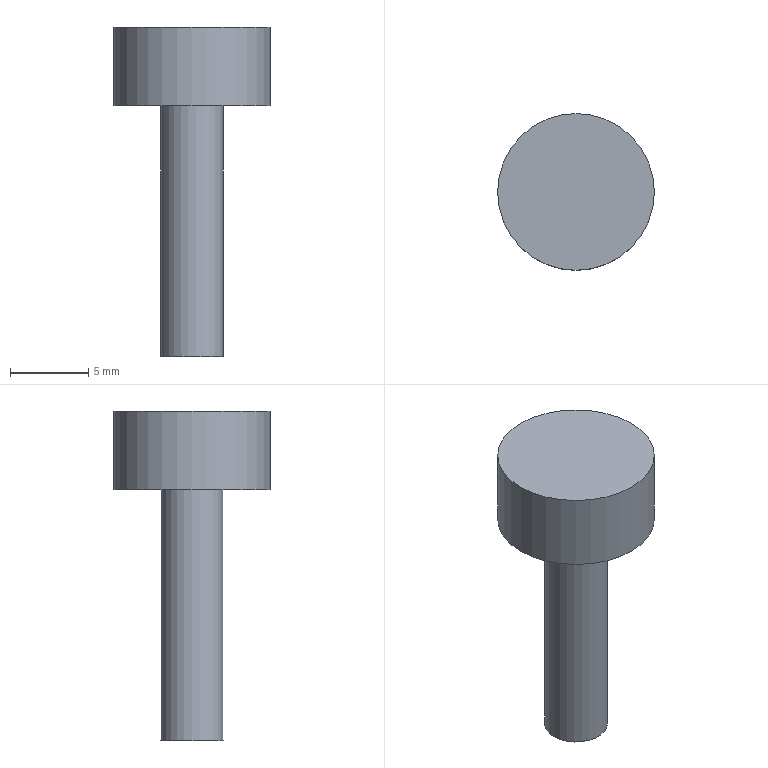Part | NX | features CYLINDER 2, DATUM_CSYS 1 | 1 solid | 5 faces | box 10 x 10 x 21 mm | volume 593.761 mm3 | plane 3 | cylinder 2 | commonest cylinder face diameters 4 x1 10 x1
STEP:
#1=CARTESIAN_POINT('',(2.,0.,0.));
#2=VERTEX_POINT('',#1);
#3=CARTESIAN_POINT('',(0.,0.,0.));
#4=DIRECTION('',(0.,0.,1.));
#5=DIRECTION('',(1.,0.,0.));
#6=AXIS2_PLACEMENT_3D('',#3,#4,#5);
#7=CIRCLE('',#6,2.);
#8=EDGE_CURVE('',#2,#2,#7,.T.);
#9=ORIENTED_EDGE('',*,*,#8,.F.);
#10=EDGE_LOOP('',(#9));
#11=FACE_BOUND('',#10,.T.);
#12=CARTESIAN_POINT('',(0.,0.,0.));
#13=DIRECTION('',(0.,0.,-1.));
#14=DIRECTION('',(-1.,0.,0.));
#15=AXIS2_PLACEMENT_3D('',#12,#13,#14);
#16=PLANE('',#15);
#17=ADVANCED_FACE('',(#11),#16,.T.);
#18=CARTESIAN_POINT('',(2.,0.,16.));
#19=VERTEX_POINT('',#18);
#20=CARTESIAN_POINT('',(0.,0.,16.));
#21=DIRECTION('',(0.,0.,-1.));
#22=DIRECTION('',(1.,0.,0.));
#23=AXIS2_PLACEMENT_3D('',#20,#21,#22);
#24=CIRCLE('',#23,2.);
#25=EDGE_CURVE('',#19,#19,#24,.T.);
#26=ORIENTED_EDGE('',*,*,#25,.T.);
#27=EDGE_LOOP('',(#26));
#28=FACE_BOUND('',#27,.T.);
#29=ORIENTED_EDGE('',*,*,#8,.T.);
#30=EDGE_LOOP('',(#29));
#31=FACE_BOUND('',#30,.T.);
#32=CARTESIAN_POINT('',(0.,0.,0.));
#33=DIRECTION('',(0.,0.,1.));
#34=DIRECTION('',(1.,0.,0.));
#35=AXIS2_PLACEMENT_3D('',#32,#33,#34);
#36=CYLINDRICAL_SURFACE('',#35,2.);
#37=ADVANCED_FACE('',(#28,#31),#36,.T.);
#38=CARTESIAN_POINT('',(5.,0.,21.));
#39=VERTEX_POINT('',#38);
#40=CARTESIAN_POINT('',(0.,0.,21.));
#41=DIRECTION('',(0.,0.,-1.));
#42=DIRECTION('',(1.,0.,0.));
#43=AXIS2_PLACEMENT_3D('',#40,#41,#42);
#44=CIRCLE('',#43,5.);
#45=EDGE_CURVE('',#39,#39,#44,.T.);
#46=ORIENTED_EDGE('',*,*,#45,.F.);
#47=EDGE_LOOP('',(#46));
#48=FACE_BOUND('',#47,.T.);
#49=CARTESIAN_POINT('',(0.,0.,21.));
#50=DIRECTION('',(0.,0.,1.));
#51=DIRECTION('',(1.,0.,0.));
#52=AXIS2_PLACEMENT_3D('',#49,#50,#51);
#53=PLANE('',#52);
#54=ADVANCED_FACE('',(#48),#53,.T.);
#55=ORIENTED_EDGE('',*,*,#25,.F.);
#56=EDGE_LOOP('',(#55));
#57=FACE_BOUND('',#56,.T.);
#58=CARTESIAN_POINT('',(5.,0.,16.));
#59=VERTEX_POINT('',#58);
#60=CARTESIAN_POINT('',(0.,0.,16.));
#61=DIRECTION('',(0.,0.,1.));
#62=DIRECTION('',(1.,0.,0.));
#63=AXIS2_PLACEMENT_3D('',#60,#61,#62);
#64=CIRCLE('',#63,5.);
#65=EDGE_CURVE('',#59,#59,#64,.T.);
#66=ORIENTED_EDGE('',*,*,#65,.F.);
#67=EDGE_LOOP('',(#66));
#68=FACE_BOUND('',#67,.T.);
#69=CARTESIAN_POINT('',(0.,0.,16.));
#70=DIRECTION('',(0.,0.,-1.));
#71=DIRECTION('',(-1.,0.,0.));
#72=AXIS2_PLACEMENT_3D('',#69,#70,#71);
#73=PLANE('',#72);
#74=ADVANCED_FACE('',(#57,#68),#73,.T.);
#75=ORIENTED_EDGE('',*,*,#45,.T.);
#76=EDGE_LOOP('',(#75));
#77=FACE_BOUND('',#76,.T.);
#78=ORIENTED_EDGE('',*,*,#65,.T.);
#79=EDGE_LOOP('',(#78));
#80=FACE_BOUND('',#79,.T.);
#81=CARTESIAN_POINT('',(0.,0.,16.));
#82=DIRECTION('',(0.,0.,1.));
#83=DIRECTION('',(1.,0.,0.));
#84=AXIS2_PLACEMENT_3D('',#81,#82,#83);
#85=CYLINDRICAL_SURFACE('',#84,5.);
#86=ADVANCED_FACE('',(#77,#80),#85,.T.);
#87=CLOSED_SHELL('',(#17,#37,#54,#74,#86));
#88=MANIFOLD_SOLID_BREP('',#87);
#89=(LENGTH_UNIT()NAMED_UNIT(*)SI_UNIT(.MILLI.,.METRE.));
#90=UNCERTAINTY_MEASURE_WITH_UNIT(LENGTH_MEASURE(0.00001),#89,'','');
#91=(NAMED_UNIT(*)PLANE_ANGLE_UNIT()SI_UNIT($,.RADIAN.));
#92=(NAMED_UNIT(*)SI_UNIT($,.STERADIAN.)SOLID_ANGLE_UNIT());
#93=(GEOMETRIC_REPRESENTATION_CONTEXT(3)GLOBAL_UNCERTAINTY_ASSIGNED_CONTEXT((#90))GLOBAL_UNIT_ASSIGNED_CONTEXT((#89,#91,#92))REPRESENTATION_CONTEXT('',''));
#94=ADVANCED_BREP_SHAPE_REPRESENTATION('',(#88),#93);